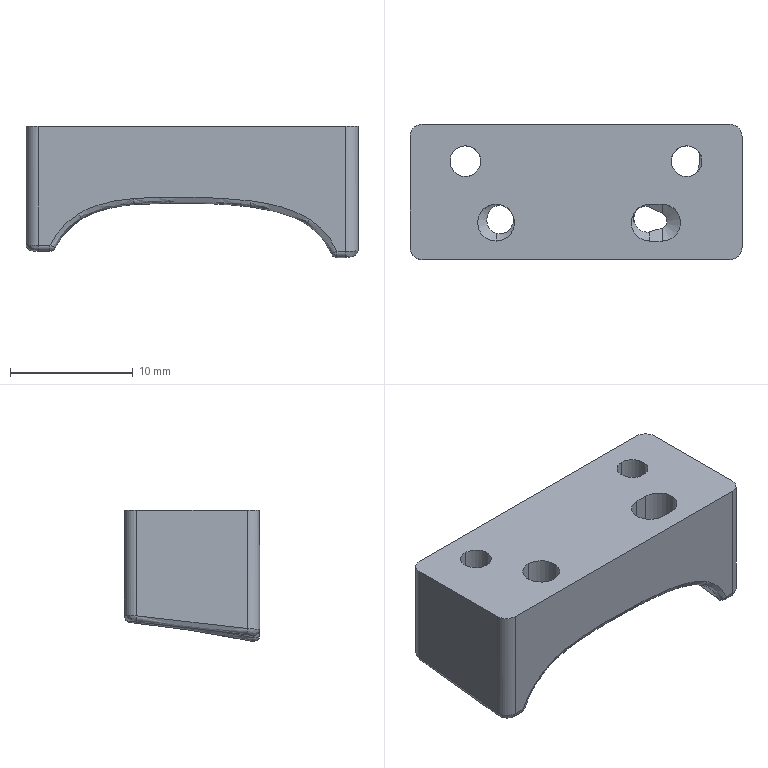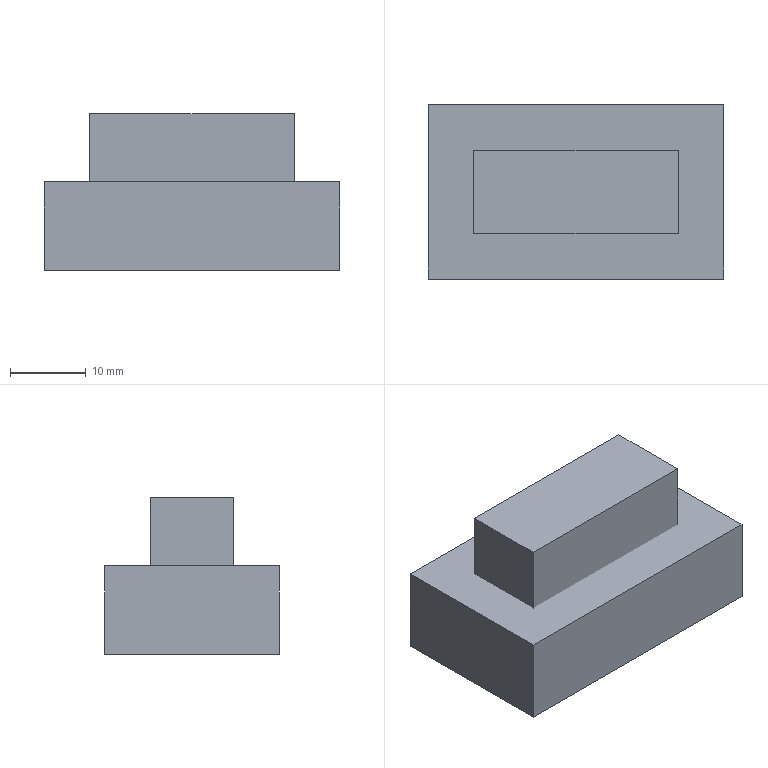CAM job | NX | 3-axis milling, drilling | part box 27 x 11 x 10.668 mm | stock box 39 x 23 x 20.668 mm
Tools:
number,name,description,diameter,corner_radius,flute_length,length,flutes
1,D50,Milling Tool-5 Parameters,50.0,0.0,50.0,75.0,2
7,D6A45,Milling Tool-5 Parameters,6.0,0.0,3.0,3.0,2
11,2.5ZT,Drilling Tool,2.5,0.0,35.0,50.0,2
5,D2,Milling Tool-5 Parameters,2.0,0.0,50.0,75.0,2
10,D10,Milling Tool-5 Parameters,10.0,0.0,50.0,75.0,2
6,D6,Milling Tool-5 Parameters,6.0,0.0,50.0,75.0,2
5,R3,Milling Tool-5 Parameters,6.0,3.0,50.0,75.0,2
Operations:
program,operation,operation_type,tool,method,geometry_group,spindle_rpm,surface_speed,feed_per_tooth,feed_cut,feed_plunge,cut_length_mm,path_length_mm,cut_time_min,machine_time_min
1-20-20-36毛胚,FLOOR_WALL,VolumeBased25DMillingOperation,D50,METHOD,A,6500.0,1286.0,0.0962,1250.0,100.0,101.0,155.0,0.0808,0.0862
1-20-20-36毛胚,DRILLING_COPY_1_COPY_1,Operation,D6A45,METHOD,A,3000.0,56.0,0.0333,200.0,0.0,18.4,131.557,0.092,0.1033
1-20-20-36毛胚,DRILLING_COPY_1_COPY_COPY_COPY_COPY_COPY_COPY,Operation,2.5ZT,METHOD,A,2000.0,15.0,0.0375,150.0,0.0,42.972,180.701,0.2865,0.3003
1-20-20-36毛胚,ADAPTIVE_MILLING,CavityMilling,D10,METHOD,A,7000.0,219.0,0.2143,3000.0,1000.0,1019.593,1094.93,0.3419,0.3494
1-20-20-36毛胚,ZLEVEL_PROFILE_COPY_COPY_1_COPY_COPY_COPY_1,ZLevelMilling,D6,METHOD,A,7000.0,219.0,0.0714,1000.0,100.0,95.026,176.363,0.095,0.1032
1-20-20-36毛胚,ZLEVEL_PROFILE_1,ZLevelMilling,D2,METHOD,A,7000.0,65.0,0.0786,1100.0,1000.0,355.343,496.859,0.327,0.3412
1-20-20-36毛胚,ZLEVEL_PROFILE_COPY_1_COPY_COPY_COPY_COPY_2_COPY_COPY_1_1_COPY_1,ZLevelMilling,D6A45,METHOD,A,7000.0,131.0,0.0714,1000.0,1000.0,101.507,475.802,0.1015,0.1389
1-20-20-36毛胚,刀补5.,ZLevelMilling,D2,METHOD,A,7000.0,65.0,0.0786,1100.0,1000.0,56.593,201.552,0.0516,0.0661
2-20-20-36毛胚,FACE_MILLING,FaceMilling,D50,METHOD,B,6500.0,1021.0,0.0962,1250.0,100.0,1330.0,2923.0,1.064,1.223
2-20-20-36毛胚,FIXED_CONTOUR,SurfaceContour,D10,METHOD,B,7000.0,0.0,0.0,2000.0,1000.0,2720.882,2774.882,1.363,1.368
2-20-20-36毛胚,FIXED_CONTOUR_COPY,SurfaceContour,R3,METHOD,B,7000.0,131.0,0.2143,3000.0,1000.0,10743.481,10903.048,3.604,3.62